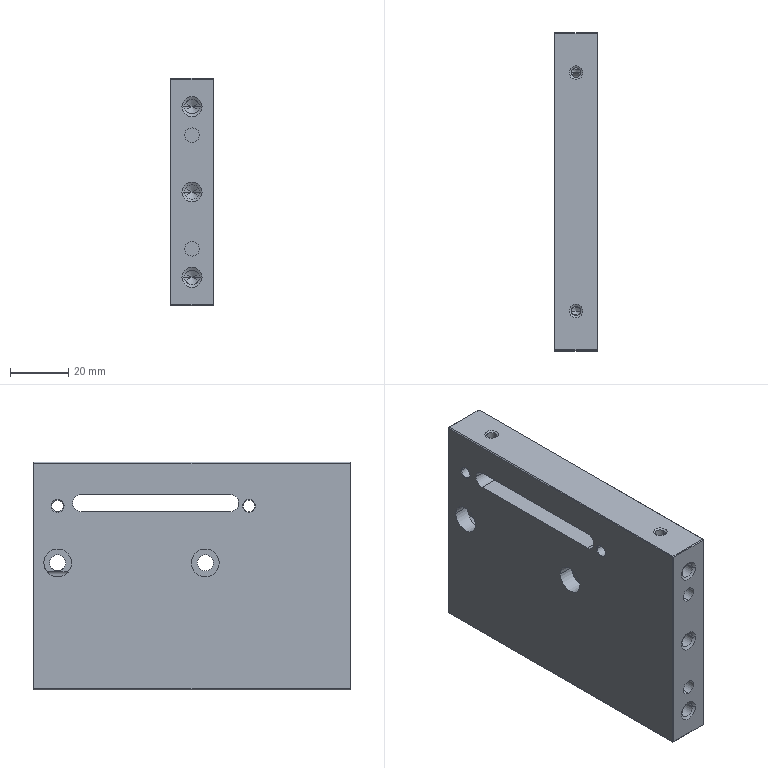Part | NX | 1 solid | 142 faces | box 15 x 109 x 78 mm | volume 117590 mm3 | cylinder 72 | cone 44 | plane 26 | commonest cylinder face diameters 5 x33 3.3 x24 4 x4 5.5 x4 9.5 x4 6 x3